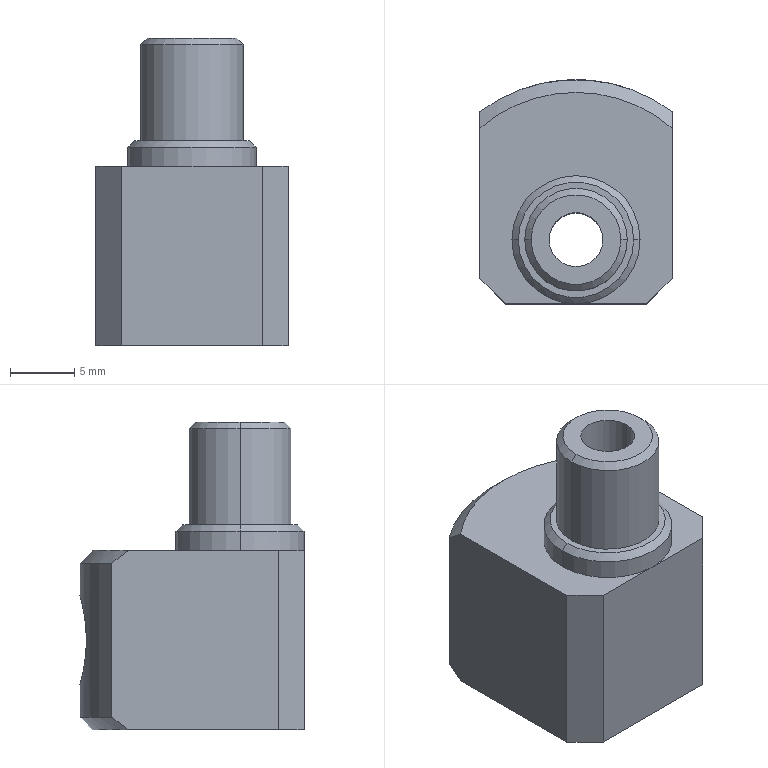Part | SolidWorks | features Chamfer 3, ICE 3, HoleWzd 2, Extrusion 1 | 1 solid | 27 faces | box 15 x 17.5 x 24 mm | volume 3225 mm3 | plane 11 | cylinder 10 | cone 6 | commonest cylinder face diameters 4.2 x3 7 x2 8 x2 10 x2 25 x1
STEP:
#1=CARTESIAN_POINT('',(3.5,0.,12.));
#2=VERTEX_POINT('',#1);
#3=CARTESIAN_POINT('',(-3.5,0.,12.));
#4=VERTEX_POINT('',#3);
#5=CARTESIAN_POINT('',(0.,0.,12.));
#6=DIRECTION('',(0.,0.,1.));
#7=DIRECTION('',(1.,0.,0.));
#8=AXIS2_PLACEMENT_3D('',#5,#6,#7);
#9=CIRCLE('',#8,3.5);
#10=EDGE_CURVE('',#2,#4,#9,.T.);
#11=ORIENTED_EDGE('',*,*,#10,.F.);
#12=CARTESIAN_POINT('',(4.,0.,11.5));
#13=VERTEX_POINT('',#12);
#14=CARTESIAN_POINT('',(3.5,0.,12.));
#15=DIRECTION('',(0.7071,0.,-0.7071));
#16=VECTOR('',#15,1000.);
#17=LINE('',#14,#16);
#18=EDGE_CURVE('',#2,#13,#17,.T.);
#19=ORIENTED_EDGE('',*,*,#18,.T.);
#20=CARTESIAN_POINT('',(-4.,0.,11.5));
#21=VERTEX_POINT('',#20);
#22=CARTESIAN_POINT('',(0.,0.,11.5));
#23=DIRECTION('',(0.,0.,-1.));
#24=DIRECTION('',(1.,0.,0.));
#25=AXIS2_PLACEMENT_3D('',#22,#23,#24);
#26=CIRCLE('',#25,4.);
#27=EDGE_CURVE('',#21,#13,#26,.T.);
#28=ORIENTED_EDGE('',*,*,#27,.F.);
#29=CARTESIAN_POINT('',(-3.5,0.,12.));
#30=DIRECTION('',(-0.7071,0.,-0.7071));
#31=VECTOR('',#30,1000.);
#32=LINE('',#29,#31);
#33=EDGE_CURVE('',#4,#21,#32,.T.);
#34=ORIENTED_EDGE('',*,*,#33,.F.);
#35=EDGE_LOOP('',(#11,#19,#28,#34));
#36=FACE_OUTER_BOUND('',#35,.T.);
#37=CARTESIAN_POINT('',(0.,0.,12.));
#38=DIRECTION('',(0.,0.,-1.));
#39=DIRECTION('',(-1.,0.,0.));
#40=AXIS2_PLACEMENT_3D('',#37,#38,#39);
#41=CONICAL_SURFACE('',#40,3.5,0.7854);
#42=ADVANCED_FACE('',(#36),#41,.T.);
#43=CARTESIAN_POINT('',(4.5,0.,4.));
#44=VERTEX_POINT('',#43);
#45=CARTESIAN_POINT('',(-4.5,0.,4.));
#46=VERTEX_POINT('',#45);
#47=CARTESIAN_POINT('',(0.,0.,4.));
#48=DIRECTION('',(0.,0.,1.));
#49=DIRECTION('',(1.,0.,0.));
#50=AXIS2_PLACEMENT_3D('',#47,#48,#49);
#51=CIRCLE('',#50,4.5);
#52=EDGE_CURVE('',#44,#46,#51,.T.);
#53=ORIENTED_EDGE('',*,*,#52,.F.);
#54=CARTESIAN_POINT('',(5.,0.,3.5));
#55=VERTEX_POINT('',#54);
#56=CARTESIAN_POINT('',(4.5,0.,4.));
#57=DIRECTION('',(0.7071,0.,-0.7071));
#58=VECTOR('',#57,1000.);
#59=LINE('',#56,#58);
#60=EDGE_CURVE('',#44,#55,#59,.T.);
#61=ORIENTED_EDGE('',*,*,#60,.T.);
#62=CARTESIAN_POINT('',(-5.,0.,3.5));
#63=VERTEX_POINT('',#62);
#64=CARTESIAN_POINT('',(0.,0.,3.5));
#65=DIRECTION('',(0.,0.,-1.));
#66=DIRECTION('',(1.,0.,0.));
#67=AXIS2_PLACEMENT_3D('',#64,#65,#66);
#68=CIRCLE('',#67,5.);
#69=EDGE_CURVE('',#63,#55,#68,.T.);
#70=ORIENTED_EDGE('',*,*,#69,.F.);
#71=CARTESIAN_POINT('',(-4.5,0.,4.));
#72=DIRECTION('',(-0.7071,0.,-0.7071));
#73=VECTOR('',#72,1000.);
#74=LINE('',#71,#73);
#75=EDGE_CURVE('',#46,#63,#74,.T.);
#76=ORIENTED_EDGE('',*,*,#75,.F.);
#77=EDGE_LOOP('',(#53,#61,#70,#76));
#78=FACE_OUTER_BOUND('',#77,.T.);
#79=CARTESIAN_POINT('',(0.,0.,4.));
#80=DIRECTION('',(0.,0.,-1.));
#81=DIRECTION('',(-1.,0.,0.));
#82=AXIS2_PLACEMENT_3D('',#79,#80,#81);
#83=CONICAL_SURFACE('',#82,4.5,0.7854);
#84=ADVANCED_FACE('',(#78),#83,.T.);
#85=CARTESIAN_POINT('',(0.,12.5,-1.5));
#86=VERTEX_POINT('',#85);
#87=CARTESIAN_POINT('',(0.,12.5,-8.5));
#88=VERTEX_POINT('',#87);
#89=CARTESIAN_POINT('',(0.,12.5,-1.5));
#90=CARTESIAN_POINT('',(-0.2291,12.5,-1.5));
#91=CARTESIAN_POINT('',(-0.4583,12.494,-1.522));
#92=CARTESIAN_POINT('',(-0.9128,12.469,-1.613));
#93=CARTESIAN_POINT('',(-1.132,12.45,-1.68));
#94=CARTESIAN_POINT('',(-1.553,12.405,-1.855));
#95=CARTESIAN_POINT('',(-1.758,12.377,-1.965));
#96=CARTESIAN_POINT('',(-2.137,12.317,-2.219));
#97=CARTESIAN_POINT('',(-2.313,12.285,-2.363));
#98=CARTESIAN_POINT('',(-2.636,12.22,-2.686));
#99=CARTESIAN_POINT('',(-2.782,12.187,-2.864));
#100=CARTESIAN_POINT('',(-3.035,12.127,-3.242));
#101=CARTESIAN_POINT('',(-3.143,12.099,-3.443));
#102=CARTESIAN_POINT('',(-3.32,12.051,-3.869));
#103=CARTESIAN_POINT('',(-3.387,12.032,-4.088));
#104=CARTESIAN_POINT('',(-3.477,12.007,-4.537));
#105=CARTESIAN_POINT('',(-3.5,12.,-4.769));
#106=CARTESIAN_POINT('',(-3.5,12.,-5.23));
#107=CARTESIAN_POINT('',(-3.477,12.007,-5.458));
#108=CARTESIAN_POINT('',(-3.388,12.032,-5.908));
#109=CARTESIAN_POINT('',(-3.32,12.051,-6.132));
#110=CARTESIAN_POINT('',(-3.145,12.098,-6.553));
#111=CARTESIAN_POINT('',(-3.037,12.126,-6.755));
#112=CARTESIAN_POINT('',(-2.782,12.187,-7.137));
#113=CARTESIAN_POINT('',(-2.636,12.22,-7.313));
#114=CARTESIAN_POINT('',(-2.316,12.285,-7.634));
#115=CARTESIAN_POINT('',(-2.138,12.317,-7.781));
#116=CARTESIAN_POINT('',(-1.757,12.377,-8.035));
#117=CARTESIAN_POINT('',(-1.557,12.404,-8.143));
#118=CARTESIAN_POINT('',(-1.135,12.45,-8.319));
#119=CARTESIAN_POINT('',(-0.9118,12.469,-8.387));
#120=CARTESIAN_POINT('',(-0.4613,12.494,-8.477));
#121=CARTESIAN_POINT('',(-0.2324,12.5,-8.5));
#122=CARTESIAN_POINT('',(0.,12.5,-8.5));
#123=B_SPLINE_CURVE_WITH_KNOTS('',3,(#89,#90,#91,#92,#93,#94,#95,#96,#97,#98,#99,#100,#101,#102,#103,#104,#105,#106,#107,#108,#109,#110,#111,#112,#113,#114,#115,#116,#117,#118,#119,#120,#121,#122),.UNSPECIFIED.,.F.,.F.,(4,2,2,2,2,2,2,2,2,2,2,2,2,2,2,2,4),(0.011,0.01169,0.01237,0.01306,0.01375,0.01443,0.01512,0.01581,0.0165,0.01718,0.01787,0.01856,0.01924,0.01993,0.02062,0.02131,0.02199),.UNSPECIFIED.);
#124=EDGE_CURVE('',#86,#88,#123,.T.);
#125=ORIENTED_EDGE('',*,*,#124,.F.);
#126=CARTESIAN_POINT('',(0.,2.1,-1.5));
#127=VERTEX_POINT('',#126);
#128=CARTESIAN_POINT('',(0.,0.,-1.5));
#129=DIRECTION('',(0.,-1.,0.));
#130=VECTOR('',#129,1000.);
#131=LINE('',#128,#130);
#132=EDGE_CURVE('',#86,#127,#131,.T.);
#133=ORIENTED_EDGE('',*,*,#132,.T.);
#134=CARTESIAN_POINT('',(-2.1,0.,-2.2));
#135=VERTEX_POINT('',#134);
#136=CARTESIAN_POINT('',(-2.1,0.,-2.2));
#137=CARTESIAN_POINT('',(-2.1,0.1429,-2.2));
#138=CARTESIAN_POINT('',(-2.086,0.2824,-2.189));
#139=CARTESIAN_POINT('',(-2.03,0.5553,-2.149));
#140=CARTESIAN_POINT('',(-1.988,0.6898,-2.119));
#141=CARTESIAN_POINT('',(-1.829,1.068,-2.013));
#142=CARTESIAN_POINT('',(-1.675,1.294,-1.92));
#143=CARTESIAN_POINT('',(-1.392,1.578,-1.787));
#144=CARTESIAN_POINT('',(-1.287,1.665,-1.743));
#145=CARTESIAN_POINT('',(-1.062,1.816,-1.663));
#146=CARTESIAN_POINT('',(-0.9435,1.881,-1.627));
#147=CARTESIAN_POINT('',(-0.6905,1.988,-1.566));
#148=CARTESIAN_POINT('',(-0.5548,2.03,-1.542));
#149=CARTESIAN_POINT('',(-0.2811,2.086,-1.509));
#150=CARTESIAN_POINT('',(-0.1418,2.1,-1.5));
#151=CARTESIAN_POINT('',(0.,2.1,-1.5));
#152=B_SPLINE_CURVE_WITH_KNOTS('',3,(#136,#137,#138,#139,#140,#141,#142,#143,#144,#145,#146,#147,#148,#149,#150,#151),.UNSPECIFIED.,.F.,.F.,(4,2,2,2,2,2,2,4),(0.,0.0004214,0.0008428,0.001686,0.002107,0.002528,0.00295,0.003371),.UNSPECIFIED.);
#153=EDGE_CURVE('',#135,#127,#152,.T.);
#154=ORIENTED_EDGE('',*,*,#153,.F.);
#155=CARTESIAN_POINT('',(-2.1,0.,-7.8));
#156=VERTEX_POINT('',#155);
#157=CARTESIAN_POINT('',(0.,0.,-5.));
#158=DIRECTION('',(0.,-1.,0.));
#159=DIRECTION('',(0.,0.,-1.));
#160=AXIS2_PLACEMENT_3D('',#157,#158,#159);
#161=CIRCLE('',#160,3.5);
#162=EDGE_CURVE('',#135,#156,#161,.T.);
#163=ORIENTED_EDGE('',*,*,#162,.T.);
#164=CARTESIAN_POINT('',(0.,2.1,-8.5));
#165=VERTEX_POINT('',#164);
#166=CARTESIAN_POINT('',(0.,2.1,-8.5));
#167=CARTESIAN_POINT('',(-0.2831,2.1,-8.5));
#168=CARTESIAN_POINT('',(-0.5647,2.041,-8.464));
#169=CARTESIAN_POINT('',(-1.073,1.826,-8.342));
#170=CARTESIAN_POINT('',(-1.3,1.671,-8.256));
#171=CARTESIAN_POINT('',(-1.583,1.387,-8.123));
#172=CARTESIAN_POINT('',(-1.669,1.282,-8.078));
#173=CARTESIAN_POINT('',(-1.819,1.059,-7.992));
#174=CARTESIAN_POINT('',(-1.882,0.9407,-7.951));
#175=CARTESIAN_POINT('',(-1.988,0.6903,-7.881));
#176=CARTESIAN_POINT('',(-2.03,0.556,-7.851));
#177=CARTESIAN_POINT('',(-2.086,0.2824,-7.811));
#178=CARTESIAN_POINT('',(-2.1,0.1428,-7.8));
#179=CARTESIAN_POINT('',(-2.1,0.,-7.8));
#180=B_SPLINE_CURVE_WITH_KNOTS('',3,(#166,#167,#168,#169,#170,#171,#172,#173,#174,#175,#176,#177,#178,#179),.UNSPECIFIED.,.F.,.F.,(4,2,2,2,2,2,4),(0.003371,0.004212,0.005053,0.005473,0.005894,0.006314,0.006735),.UNSPECIFIED.);
#181=EDGE_CURVE('',#165,#156,#180,.T.);
#182=ORIENTED_EDGE('',*,*,#181,.F.);
#183=CARTESIAN_POINT('',(0.,0.,-8.5));
#184=DIRECTION('',(0.,-1.,0.));
#185=VECTOR('',#184,1000.);
#186=LINE('',#183,#185);
#187=EDGE_CURVE('',#88,#165,#186,.T.);
#188=ORIENTED_EDGE('',*,*,#187,.F.);
#189=EDGE_LOOP('',(#125,#133,#154,#163,#182,#188));
#190=FACE_OUTER_BOUND('',#189,.T.);
#191=CARTESIAN_POINT('',(0.,0.,-5.));
#192=DIRECTION('',(0.,-1.,0.));
#193=DIRECTION('',(0.,0.,-1.));
#194=AXIS2_PLACEMENT_3D('',#191,#192,#193);
#195=CYLINDRICAL_SURFACE('',#194,3.5);
#196=ADVANCED_FACE('',(#190),#195,.F.);
#197=ORIENTED_EDGE('',*,*,#69,.T.);
#198=CARTESIAN_POINT('',(5.,0.,2.));
#199=VERTEX_POINT('',#198);
#200=CARTESIAN_POINT('',(5.,0.,4.));
#201=DIRECTION('',(0.,0.,-1.));
#202=VECTOR('',#201,1000.);
#203=LINE('',#200,#202);
#204=EDGE_CURVE('',#55,#199,#203,.T.);
#205=ORIENTED_EDGE('',*,*,#204,.T.);
#206=CARTESIAN_POINT('',(-5.,0.,2.));
#207=VERTEX_POINT('',#206);
#208=CARTESIAN_POINT('',(0.,0.,2.));
#209=DIRECTION('',(0.,0.,1.));
#210=DIRECTION('',(1.,0.,0.));
#211=AXIS2_PLACEMENT_3D('',#208,#209,#210);
#212=CIRCLE('',#211,5.);
#213=EDGE_CURVE('',#199,#207,#212,.T.);
#214=ORIENTED_EDGE('',*,*,#213,.T.);
#215=CARTESIAN_POINT('',(-5.,0.,4.));
#216=DIRECTION('',(0.,0.,-1.));
#217=VECTOR('',#216,1000.);
#218=LINE('',#215,#217);
#219=EDGE_CURVE('',#63,#207,#218,.T.);
#220=ORIENTED_EDGE('',*,*,#219,.F.);
#221=EDGE_LOOP('',(#197,#205,#214,#220));
#222=FACE_OUTER_BOUND('',#221,.T.);
#223=CARTESIAN_POINT('',(0.,0.,4.));
#224=DIRECTION('',(0.,0.,-1.));
#225=DIRECTION('',(-1.,0.,0.));
#226=AXIS2_PLACEMENT_3D('',#223,#224,#225);
#227=CYLINDRICAL_SURFACE('',#226,5.);
#228=ADVANCED_FACE('',(#222),#227,.T.);
#229=CARTESIAN_POINT('',(2.1,0.,12.));
#230=VERTEX_POINT('',#229);
#231=CARTESIAN_POINT('',(-2.1,0.,12.));
#232=VERTEX_POINT('',#231);
#233=CARTESIAN_POINT('',(0.,0.,12.));
#234=DIRECTION('',(0.,0.,-1.));
#235=DIRECTION('',(-1.,0.,0.));
#236=AXIS2_PLACEMENT_3D('',#233,#234,#235);
#237=CIRCLE('',#236,2.1);
#238=EDGE_CURVE('',#230,#232,#237,.T.);
#239=ORIENTED_EDGE('',*,*,#238,.F.);
#240=CARTESIAN_POINT('',(2.1,0.,-2.2));
#241=VERTEX_POINT('',#240);
#242=CARTESIAN_POINT('',(2.1,0.,-12.));
#243=DIRECTION('',(0.,0.,-1.));
#244=VECTOR('',#243,1000.);
#245=LINE('',#242,#244);
#246=EDGE_CURVE('',#230,#241,#245,.T.);
#247=ORIENTED_EDGE('',*,*,#246,.T.);
#248=CARTESIAN_POINT('',(2.1,0.,-7.8));
#249=VERTEX_POINT('',#248);
#250=CARTESIAN_POINT('',(2.1,0.,-12.));
#251=DIRECTION('',(0.,0.,-1.));
#252=VECTOR('',#251,1000.);
#253=LINE('',#250,#252);
#254=EDGE_CURVE('',#241,#249,#253,.T.);
#255=ORIENTED_EDGE('',*,*,#254,.T.);
#256=CARTESIAN_POINT('',(2.1,0.,-12.));
#257=VERTEX_POINT('',#256);
#258=CARTESIAN_POINT('',(2.1,0.,-12.));
#259=DIRECTION('',(0.,0.,-1.));
#260=VECTOR('',#259,1000.);
#261=LINE('',#258,#260);
#262=EDGE_CURVE('',#249,#257,#261,.T.);
#263=ORIENTED_EDGE('',*,*,#262,.T.);
#264=CARTESIAN_POINT('',(-2.1,0.,-12.));
#265=VERTEX_POINT('',#264);
#266=CARTESIAN_POINT('',(0.,0.,-12.));
#267=DIRECTION('',(0.,0.,-1.));
#268=DIRECTION('',(-1.,0.,0.));
#269=AXIS2_PLACEMENT_3D('',#266,#267,#268);
#270=CIRCLE('',#269,2.1);
#271=EDGE_CURVE('',#257,#265,#270,.T.);
#272=ORIENTED_EDGE('',*,*,#271,.T.);
#273=CARTESIAN_POINT('',(-2.1,0.,-12.));
#274=DIRECTION('',(0.,0.,-1.));
#275=VECTOR('',#274,1000.);
#276=LINE('',#273,#275);
#277=EDGE_CURVE('',#156,#265,#276,.T.);
#278=ORIENTED_EDGE('',*,*,#277,.F.);
#279=CARTESIAN_POINT('',(-2.1,0.,-12.));
#280=DIRECTION('',(0.,0.,1.));
#281=VECTOR('',#280,1000.);
#282=LINE('',#279,#281);
#283=EDGE_CURVE('',#156,#135,#282,.T.);
#284=ORIENTED_EDGE('',*,*,#283,.T.);
#285=CARTESIAN_POINT('',(-2.1,0.,-12.));
#286=DIRECTION('',(0.,0.,-1.));
#287=VECTOR('',#286,1000.);
#288=LINE('',#285,#287);
#289=EDGE_CURVE('',#232,#135,#288,.T.);
#290=ORIENTED_EDGE('',*,*,#289,.F.);
#291=EDGE_LOOP('',(#239,#247,#255,#263,#272,#278,#284,#290));
#292=FACE_OUTER_BOUND('',#291,.T.);
#293=CARTESIAN_POINT('',(0.,0.,-12.));
#294=DIRECTION('',(0.,0.,-1.));
#295=DIRECTION('',(-1.,0.,0.));
#296=AXIS2_PLACEMENT_3D('',#293,#294,#295);
#297=CYLINDRICAL_SURFACE('',#296,2.1);
#298=ADVANCED_FACE('',(#292),#297,.F.);
#299=ORIENTED_EDGE('',*,*,#246,.F.);
#300=CARTESIAN_POINT('',(0.,0.,12.));
#301=DIRECTION('',(0.,0.,-1.));
#302=DIRECTION('',(-1.,0.,0.));
#303=AXIS2_PLACEMENT_3D('',#300,#301,#302);
#304=CIRCLE('',#303,2.1);
#305=EDGE_CURVE('',#232,#230,#304,.T.);
#306=ORIENTED_EDGE('',*,*,#305,.F.);
#307=ORIENTED_EDGE('',*,*,#289,.T.);
#308=ORIENTED_EDGE('',*,*,#153,.T.);
#309=CARTESIAN_POINT('',(0.,2.1,-1.5));
#310=CARTESIAN_POINT('',(0.2831,2.1,-1.5));
#311=CARTESIAN_POINT('',(0.5647,2.041,-1.536));
#312=CARTESIAN_POINT('',(1.073,1.826,-1.658));
#313=CARTESIAN_POINT('',(1.3,1.671,-1.744));
#314=CARTESIAN_POINT('',(1.583,1.387,-1.877));
#315=CARTESIAN_POINT('',(1.669,1.282,-1.922));
#316=CARTESIAN_POINT('',(1.819,1.059,-2.008));
#317=CARTESIAN_POINT('',(1.882,0.9407,-2.049));
#318=CARTESIAN_POINT('',(1.988,0.6903,-2.119));
#319=CARTESIAN_POINT('',(2.03,0.556,-2.149));
#320=CARTESIAN_POINT('',(2.086,0.2824,-2.189));
#321=CARTESIAN_POINT('',(2.1,0.1428,-2.2));
#322=CARTESIAN_POINT('',(2.1,0.,-2.2));
#323=B_SPLINE_CURVE_WITH_KNOTS('',3,(#309,#310,#311,#312,#313,#314,#315,#316,#317,#318,#319,#320,#321,#322),.UNSPECIFIED.,.F.,.F.,(4,2,2,2,2,2,4),(0.003371,0.004212,0.005053,0.005473,0.005894,0.006314,0.006735),.UNSPECIFIED.);
#324=EDGE_CURVE('',#127,#241,#323,.T.);
#325=ORIENTED_EDGE('',*,*,#324,.T.);
#326=EDGE_LOOP('',(#299,#306,#307,#308,#325));
#327=FACE_OUTER_BOUND('',#326,.T.);
#328=CARTESIAN_POINT('',(0.,0.,-12.));
#329=DIRECTION('',(0.,0.,-1.));
#330=DIRECTION('',(-1.,0.,0.));
#331=AXIS2_PLACEMENT_3D('',#328,#329,#330);
#332=CYLINDRICAL_SURFACE('',#331,2.1);
#333=ADVANCED_FACE('',(#327),#332,.F.);
#334=CARTESIAN_POINT('',(-4.,0.,4.));
#335=VERTEX_POINT('',#334);
#336=CARTESIAN_POINT('',(4.,0.,4.));
#337=VERTEX_POINT('',#336);
#338=CARTESIAN_POINT('',(0.,0.,4.));
#339=DIRECTION('',(0.,0.,-1.));
#340=DIRECTION('',(1.,0.,0.));
#341=AXIS2_PLACEMENT_3D('',#338,#339,#340);
#342=CIRCLE('',#341,4.);
#343=EDGE_CURVE('',#335,#337,#342,.T.);
#344=ORIENTED_EDGE('',*,*,#343,.F.);
#345=CARTESIAN_POINT('',(-4.,0.,2.));
#346=DIRECTION('',(0.,0.,1.));
#347=VECTOR('',#346,1000.);
#348=LINE('',#345,#347);
#349=EDGE_CURVE('',#335,#21,#348,.T.);
#350=ORIENTED_EDGE('',*,*,#349,.T.);
#351=ORIENTED_EDGE('',*,*,#27,.T.);
#352=CARTESIAN_POINT('',(4.,0.,2.));
#353=DIRECTION('',(0.,0.,1.));
#354=VECTOR('',#353,1000.);
#355=LINE('',#352,#354);
#356=EDGE_CURVE('',#337,#13,#355,.T.);
#357=ORIENTED_EDGE('',*,*,#356,.F.);
#358=EDGE_LOOP('',(#344,#350,#351,#357));
#359=FACE_OUTER_BOUND('',#358,.T.);
#360=CARTESIAN_POINT('',(0.,0.,2.));
#361=DIRECTION('',(0.,0.,1.));
#362=DIRECTION('',(1.,0.,0.));
#363=AXIS2_PLACEMENT_3D('',#360,#361,#362);
#364=CYLINDRICAL_SURFACE('',#363,4.);
#365=ADVANCED_FACE('',(#359),#364,.T.);
#366=CARTESIAN_POINT('',(7.5,-3.,2.));
#367=VERTEX_POINT('',#366);
#368=CARTESIAN_POINT('',(7.5,8.718,2.));
#369=VERTEX_POINT('',#368);
#370=CARTESIAN_POINT('',(7.5,0.,2.));
#371=DIRECTION('',(0.,1.,0.));
#372=VECTOR('',#371,1000.);
#373=LINE('',#370,#372);
#374=EDGE_CURVE('',#367,#369,#373,.T.);
#375=ORIENTED_EDGE('',*,*,#374,.T.);
#376=CARTESIAN_POINT('',(-7.5,8.718,2.));
#377=VERTEX_POINT('',#376);
#378=CARTESIAN_POINT('',(0.,0.,2.));
#379=DIRECTION('',(0.,0.,1.));
#380=DIRECTION('',(1.,0.,0.));
#381=AXIS2_PLACEMENT_3D('',#378,#379,#380);
#382=CIRCLE('',#381,11.5);
#383=EDGE_CURVE('',#369,#377,#382,.T.);
#384=ORIENTED_EDGE('',*,*,#383,.T.);
#385=CARTESIAN_POINT('',(-7.5,-3.,2.));
#386=VERTEX_POINT('',#385);
#387=CARTESIAN_POINT('',(-7.5,0.,2.));
#388=DIRECTION('',(0.,-1.,0.));
#389=VECTOR('',#388,1000.);
#390=LINE('',#387,#389);
#391=EDGE_CURVE('',#377,#386,#390,.T.);
#392=ORIENTED_EDGE('',*,*,#391,.T.);
#393=CARTESIAN_POINT('',(-5.5,-5.,2.));
#394=VERTEX_POINT('',#393);
#395=CARTESIAN_POINT('',(-5.25,-5.25,2.));
#396=DIRECTION('',(0.7071,-0.7071,0.));
#397=VECTOR('',#396,1000.);
#398=LINE('',#395,#397);
#399=EDGE_CURVE('',#386,#394,#398,.T.);
#400=ORIENTED_EDGE('',*,*,#399,.T.);
#401=CARTESIAN_POINT('',(0.,-5.,2.));
#402=VERTEX_POINT('',#401);
#403=CARTESIAN_POINT('',(0.,-5.,2.));
#404=DIRECTION('',(1.,0.,0.));
#405=VECTOR('',#404,1000.);
#406=LINE('',#403,#405);
#407=EDGE_CURVE('',#394,#402,#406,.T.);
#408=ORIENTED_EDGE('',*,*,#407,.T.);
#409=CARTESIAN_POINT('',(0.,0.,2.));
#410=DIRECTION('',(0.,0.,1.));
#411=DIRECTION('',(1.,0.,0.));
#412=AXIS2_PLACEMENT_3D('',#409,#410,#411);
#413=CIRCLE('',#412,5.);
#414=EDGE_CURVE('',#207,#402,#413,.T.);
#415=ORIENTED_EDGE('',*,*,#414,.F.);
#416=ORIENTED_EDGE('',*,*,#213,.F.);
#417=CARTESIAN_POINT('',(0.,0.,2.));
#418=DIRECTION('',(0.,0.,1.));
#419=DIRECTION('',(1.,0.,0.));
#420=AXIS2_PLACEMENT_3D('',#417,#418,#419);
#421=CIRCLE('',#420,5.);
#422=EDGE_CURVE('',#402,#199,#421,.T.);
#423=ORIENTED_EDGE('',*,*,#422,.F.);
#424=CARTESIAN_POINT('',(5.5,-5.,2.));
#425=VERTEX_POINT('',#424);
#426=CARTESIAN_POINT('',(0.,-5.,2.));
#427=DIRECTION('',(1.,0.,0.));
#428=VECTOR('',#427,1000.);
#429=LINE('',#426,#428);
#430=EDGE_CURVE('',#402,#425,#429,.T.);
#431=ORIENTED_EDGE('',*,*,#430,.T.);
#432=CARTESIAN_POINT('',(5.25,-5.25,2.));
#433=DIRECTION('',(0.7071,0.7071,0.));
#434=VECTOR('',#433,1000.);
#435=LINE('',#432,#434);
#436=EDGE_CURVE('',#425,#367,#435,.T.);
#437=ORIENTED_EDGE('',*,*,#436,.T.);
#438=EDGE_LOOP('',(#375,#384,#392,#400,#408,#415,#416,#423,#431,#437));
#439=FACE_OUTER_BOUND('',#438,.T.);
#440=CARTESIAN_POINT('',(0.,0.,2.));
#441=DIRECTION('',(0.,0.,1.));
#442=DIRECTION('',(1.,0.,0.));
#443=AXIS2_PLACEMENT_3D('',#440,#441,#442);
#444=PLANE('',#443);
#445=ADVANCED_FACE('',(#439),#444,.T.);
#446=CARTESIAN_POINT('',(0.,12.5,-8.5));
#447=CARTESIAN_POINT('',(0.2325,12.5,-8.5));
#448=CARTESIAN_POINT('',(0.4609,12.494,-8.477));
#449=CARTESIAN_POINT('',(0.9099,12.469,-8.387));
#450=CARTESIAN_POINT('',(1.133,12.45,-8.32));
#451=CARTESIAN_POINT('',(1.556,12.405,-8.143));
#452=CARTESIAN_POINT('',(1.757,12.377,-8.036));
#453=CARTESIAN_POINT('',(2.136,12.318,-7.782));
#454=CARTESIAN_POINT('',(2.315,12.285,-7.635));
#455=CARTESIAN_POINT('',(2.636,12.22,-7.313));
#456=CARTESIAN_POINT('',(2.781,12.187,-7.138));
#457=CARTESIAN_POINT('',(3.037,12.126,-6.756));
#458=CARTESIAN_POINT('',(3.144,12.098,-6.554));
#459=CARTESIAN_POINT('',(3.319,12.052,-6.133));
#460=CARTESIAN_POINT('',(3.387,12.032,-5.911));
#461=CARTESIAN_POINT('',(3.477,12.007,-5.459));
#462=CARTESIAN_POINT('',(3.5,12.,-5.231));
#463=CARTESIAN_POINT('',(3.5,12.,-4.772));
#464=CARTESIAN_POINT('',(3.477,12.007,-4.539));
#465=CARTESIAN_POINT('',(3.387,12.032,-4.089));
#466=CARTESIAN_POINT('',(3.321,12.051,-3.87));
#467=CARTESIAN_POINT('',(3.144,12.099,-3.445));
#468=CARTESIAN_POINT('',(3.035,12.127,-3.242));
#469=CARTESIAN_POINT('',(2.782,12.187,-2.864));
#470=CARTESIAN_POINT('',(2.636,12.22,-2.686));
#471=CARTESIAN_POINT('',(2.312,12.285,-2.363));
#472=CARTESIAN_POINT('',(2.137,12.317,-2.219));
#473=CARTESIAN_POINT('',(1.759,12.377,-1.965));
#474=CARTESIAN_POINT('',(1.554,12.405,-1.855));
#475=CARTESIAN_POINT('',(1.131,12.451,-1.68));
#476=CARTESIAN_POINT('',(0.913,12.469,-1.613));
#477=CARTESIAN_POINT('',(0.4615,12.494,-1.523));
#478=CARTESIAN_POINT('',(0.2291,12.5,-1.5));
#479=CARTESIAN_POINT('',(0.,12.5,-1.5));
#480=B_SPLINE_CURVE_WITH_KNOTS('',3,(#446,#447,#448,#449,#450,#451,#452,#453,#454,#455,#456,#457,#458,#459,#460,#461,#462,#463,#464,#465,#466,#467,#468,#469,#470,#471,#472,#473,#474,#475,#476,#477,#478,#479),.UNSPECIFIED.,.F.,.F.,(4,2,2,2,2,2,2,2,2,2,2,2,2,2,2,2,4),(0.,0.0006874,0.001375,0.002062,0.002749,0.003437,0.004124,0.004812,0.005499,0.006186,0.006874,0.007561,0.008248,0.008936,0.009623,0.01031,0.011),.UNSPECIFIED.);
#481=EDGE_CURVE('',#88,#86,#480,.T.);
#482=ORIENTED_EDGE('',*,*,#481,.T.);
#483=ORIENTED_EDGE('',*,*,#124,.T.);
#484=EDGE_LOOP('',(#482,#483));
#485=FACE_BOUND('',#484,.T.);
#486=CARTESIAN_POINT('',(-7.5,10.,1.));
#487=VERTEX_POINT('',#486);
#488=CARTESIAN_POINT('',(-7.5,10.,-11.));
#489=VERTEX_POINT('',#488);
#490=CARTESIAN_POINT('',(-7.5,10.,12.));
#491=DIRECTION('',(0.,0.,-1.));
#492=VECTOR('',#491,1000.);
#493=LINE('',#490,#492);
#494=EDGE_CURVE('',#487,#489,#493,.T.);
#495=ORIENTED_EDGE('',*,*,#494,.F.);
#496=CARTESIAN_POINT('',(7.5,10.,1.));
#497=VERTEX_POINT('',#496);
#498=CARTESIAN_POINT('',(0.,0.,1.));
#499=DIRECTION('',(0.,0.,-1.));
#500=DIRECTION('',(1.,0.,0.));
#501=AXIS2_PLACEMENT_3D('',#498,#499,#500);
#502=CIRCLE('',#501,12.5);
#503=EDGE_CURVE('',#487,#497,#502,.T.);
#504=ORIENTED_EDGE('',*,*,#503,.T.);
#505=CARTESIAN_POINT('',(7.5,10.,-11.));
#506=VERTEX_POINT('',#505);
#507=CARTESIAN_POINT('',(7.5,10.,12.));
#508=DIRECTION('',(0.,0.,1.));
#509=VECTOR('',#508,1000.);
#510=LINE('',#507,#509);
#511=EDGE_CURVE('',#506,#497,#510,.T.);
#512=ORIENTED_EDGE('',*,*,#511,.F.);
#513=CARTESIAN_POINT('',(0.,0.,-11.));
#514=DIRECTION('',(0.,0.,1.));
#515=DIRECTION('',(1.,0.,0.));
#516=AXIS2_PLACEMENT_3D('',#513,#514,#515);
#517=CIRCLE('',#516,12.5);
#518=EDGE_CURVE('',#506,#489,#517,.T.);
#519=ORIENTED_EDGE('',*,*,#518,.T.);
#520=EDGE_LOOP('',(#495,#504,#512,#519));
#521=FACE_OUTER_BOUND('',#520,.T.);
#522=CARTESIAN_POINT('',(0.,0.,12.));
#523=DIRECTION('',(0.,0.,-1.));
#524=DIRECTION('',(-1.,0.,0.));
#525=AXIS2_PLACEMENT_3D('',#522,#523,#524);
#526=CYLINDRICAL_SURFACE('',#525,12.5);
#527=ADVANCED_FACE('',(#485,#521),#526,.T.);
#528=CARTESIAN_POINT('',(0.,0.,-12.));
#529=DIRECTION('',(0.,0.,-1.));
#530=DIRECTION('',(-1.,0.,0.));
#531=AXIS2_PLACEMENT_3D('',#528,#529,#530);
#532=CIRCLE('',#531,2.1);
#533=EDGE_CURVE('',#265,#257,#532,.T.);
#534=ORIENTED_EDGE('',*,*,#533,.F.);
#535=ORIENTED_EDGE('',*,*,#271,.F.);
#536=EDGE_LOOP('',(#534,#535));
#537=FACE_BOUND('',#536,.T.);
#538=CARTESIAN_POINT('',(-7.5,-3.,-12.));
#539=VERTEX_POINT('',#538);
#540=CARTESIAN_POINT('',(-7.5,8.718,-12.));
#541=VERTEX_POINT('',#540);
#542=CARTESIAN_POINT('',(-7.5,15.,-12.));
#543=DIRECTION('',(0.,1.,0.));
#544=VECTOR('',#543,1000.);
#545=LINE('',#542,#544);
#546=EDGE_CURVE('',#539,#541,#545,.T.);
#547=ORIENTED_EDGE('',*,*,#546,.T.);
#548=CARTESIAN_POINT('',(7.5,8.718,-12.));
#549=VERTEX_POINT('',#548);
#550=CARTESIAN_POINT('',(0.,0.,-12.));
#551=DIRECTION('',(0.,0.,-1.));
#552=DIRECTION('',(1.,0.,0.));
#553=AXIS2_PLACEMENT_3D('',#550,#551,#552);
#554=CIRCLE('',#553,11.5);
#555=EDGE_CURVE('',#541,#549,#554,.T.);
#556=ORIENTED_EDGE('',*,*,#555,.T.);
#557=CARTESIAN_POINT('',(7.5,-3.,-12.));
#558=VERTEX_POINT('',#557);
#559=CARTESIAN_POINT('',(7.5,15.,-12.));
#560=DIRECTION('',(0.,-1.,0.));
#561=VECTOR('',#560,1000.);
#562=LINE('',#559,#561);
#563=EDGE_CURVE('',#549,#558,#562,.T.);
#564=ORIENTED_EDGE('',*,*,#563,.T.);
#565=CARTESIAN_POINT('',(5.5,-5.,-12.));
#566=VERTEX_POINT('',#565);
#567=CARTESIAN_POINT('',(7.5,-3.,-12.));
#568=DIRECTION('',(-0.7071,-0.7071,0.));
#569=VECTOR('',#568,1000.);
#570=LINE('',#567,#569);
#571=EDGE_CURVE('',#558,#566,#570,.T.);
#572=ORIENTED_EDGE('',*,*,#571,.T.);
#573=CARTESIAN_POINT('',(-5.5,-5.,-12.));
#574=VERTEX_POINT('',#573);
#575=CARTESIAN_POINT('',(7.5,-5.,-12.));
#576=DIRECTION('',(-1.,0.,0.));
#577=VECTOR('',#576,1000.);
#578=LINE('',#575,#577);
#579=EDGE_CURVE('',#566,#574,#578,.T.);
#580=ORIENTED_EDGE('',*,*,#579,.T.);
#581=CARTESIAN_POINT('',(-5.5,-5.,-12.));
#582=DIRECTION('',(-0.7071,0.7071,0.));
#583=VECTOR('',#582,1000.);
#584=LINE('',#581,#583);
#585=EDGE_CURVE('',#574,#539,#584,.T.);
#586=ORIENTED_EDGE('',*,*,#585,.T.);
#587=EDGE_LOOP('',(#547,#556,#564,#572,#580,#586));
#588=FACE_OUTER_BOUND('',#587,.T.);
#589=CARTESIAN_POINT('',(0.,0.,-12.));
#590=DIRECTION('',(0.,0.,1.));
#591=DIRECTION('',(1.,0.,0.));
#592=AXIS2_PLACEMENT_3D('',#589,#590,#591);
#593=PLANE('',#592);
#594=ADVANCED_FACE('',(#537,#588),#593,.F.);
#595=ORIENTED_EDGE('',*,*,#349,.F.);
#596=CARTESIAN_POINT('',(0.,0.,4.));
#597=DIRECTION('',(0.,0.,-1.));
#598=DIRECTION('',(1.,0.,0.));
#599=AXIS2_PLACEMENT_3D('',#596,#597,#598);
#600=CIRCLE('',#599,4.);
#601=EDGE_CURVE('',#337,#335,#600,.T.);
#602=ORIENTED_EDGE('',*,*,#601,.F.);
#603=ORIENTED_EDGE('',*,*,#356,.T.);
#604=CARTESIAN_POINT('',(0.,0.,11.5));
#605=DIRECTION('',(0.,0.,-1.));
#606=DIRECTION('',(1.,0.,0.));
#607=AXIS2_PLACEMENT_3D('',#604,#605,#606);
#608=CIRCLE('',#607,4.);
#609=EDGE_CURVE('',#13,#21,#608,.T.);
#610=ORIENTED_EDGE('',*,*,#609,.T.);
#611=EDGE_LOOP('',(#595,#602,#603,#610));
#612=FACE_OUTER_BOUND('',#611,.T.);
#613=CARTESIAN_POINT('',(0.,0.,2.));
#614=DIRECTION('',(0.,0.,1.));
#615=DIRECTION('',(1.,0.,0.));
#616=AXIS2_PLACEMENT_3D('',#613,#614,#615);
#617=CYLINDRICAL_SURFACE('',#616,4.);
#618=ADVANCED_FACE('',(#612),#617,.T.);
#619=CARTESIAN_POINT('',(0.,0.,12.));
#620=DIRECTION('',(0.,0.,1.));
#621=DIRECTION('',(1.,0.,0.));
#622=AXIS2_PLACEMENT_3D('',#619,#620,#621);
#623=CIRCLE('',#622,3.5);
#624=EDGE_CURVE('',#4,#2,#623,.T.);
#625=ORIENTED_EDGE('',*,*,#624,.T.);
#626=ORIENTED_EDGE('',*,*,#10,.T.);
#627=EDGE_LOOP('',(#625,#626));
#628=FACE_OUTER_BOUND('',#627,.T.);
#629=ORIENTED_EDGE('',*,*,#305,.T.);
#630=ORIENTED_EDGE('',*,*,#238,.T.);
#631=EDGE_LOOP('',(#629,#630));
#632=FACE_BOUND('',#631,.T.);
#633=CARTESIAN_POINT('',(0.,0.,12.));
#634=DIRECTION('',(0.,0.,1.));
#635=DIRECTION('',(1.,0.,0.));
#636=AXIS2_PLACEMENT_3D('',#633,#634,#635);
#637=PLANE('',#636);
#638=ADVANCED_FACE('',(#628,#632),#637,.T.);
#639=ORIENTED_EDGE('',*,*,#511,.T.);
#640=CARTESIAN_POINT('',(7.5,10.,1.));
#641=CARTESIAN_POINT('',(7.5,9.577,1.339));
#642=CARTESIAN_POINT('',(7.5,9.15,1.673));
#643=CARTESIAN_POINT('',(7.5,8.718,2.));
#644=B_SPLINE_CURVE_WITH_KNOTS('',3,(#640,#641,#642,#643),.UNSPECIFIED.,.F.,.F.,(4,4),(0.,0.001626),.UNSPECIFIED.);
#645=EDGE_CURVE('',#497,#369,#644,.T.);
#646=ORIENTED_EDGE('',*,*,#645,.T.);
#647=ORIENTED_EDGE('',*,*,#374,.F.);
#648=CARTESIAN_POINT('',(7.5,-3.,12.));
#649=DIRECTION('',(0.,0.,-1.));
#650=VECTOR('',#649,1000.);
#651=LINE('',#648,#650);
#652=EDGE_CURVE('',#367,#558,#651,.T.);
#653=ORIENTED_EDGE('',*,*,#652,.T.);
#654=ORIENTED_EDGE('',*,*,#563,.F.);
#655=CARTESIAN_POINT('',(7.5,8.718,-12.));
#656=CARTESIAN_POINT('',(7.5,9.15,-11.673));
#657=CARTESIAN_POINT('',(7.5,9.577,-11.339));
#658=CARTESIAN_POINT('',(7.5,10.,-11.));
#659=B_SPLINE_CURVE_WITH_KNOTS('',3,(#655,#656,#657,#658),.UNSPECIFIED.,.F.,.F.,(4,4),(0.,0.001626),.UNSPECIFIED.);
#660=EDGE_CURVE('',#549,#506,#659,.T.);
#661=ORIENTED_EDGE('',*,*,#660,.T.);
#662=EDGE_LOOP('',(#639,#646,#647,#653,#654,#661));
#663=FACE_OUTER_BOUND('',#662,.T.);
#664=CARTESIAN_POINT('',(7.5,15.,12.));
#665=DIRECTION('',(1.,0.,0.));
#666=DIRECTION('',(0.,1.,0.));
#667=AXIS2_PLACEMENT_3D('',#664,#665,#666);
#668=PLANE('',#667);
#669=ADVANCED_FACE('',(#663),#668,.T.);
#670=ORIENTED_EDGE('',*,*,#391,.F.);
#671=CARTESIAN_POINT('',(-7.5,8.718,2.));
#672=CARTESIAN_POINT('',(-7.5,9.15,1.673));
#673=CARTESIAN_POINT('',(-7.5,9.577,1.339));
#674=CARTESIAN_POINT('',(-7.5,10.,1.));
#675=B_SPLINE_CURVE_WITH_KNOTS('',3,(#671,#672,#673,#674),.UNSPECIFIED.,.F.,.F.,(4,4),(0.,0.001626),.UNSPECIFIED.);
#676=EDGE_CURVE('',#377,#487,#675,.T.);
#677=ORIENTED_EDGE('',*,*,#676,.T.);
#678=ORIENTED_EDGE('',*,*,#494,.T.);
#679=CARTESIAN_POINT('',(-7.5,10.,-11.));
#680=CARTESIAN_POINT('',(-7.5,9.577,-11.339));
#681=CARTESIAN_POINT('',(-7.5,9.15,-11.673));
#682=CARTESIAN_POINT('',(-7.5,8.718,-12.));
#683=B_SPLINE_CURVE_WITH_KNOTS('',3,(#679,#680,#681,#682),.UNSPECIFIED.,.F.,.F.,(4,4),(0.,0.001626),.UNSPECIFIED.);
#684=EDGE_CURVE('',#489,#541,#683,.T.);
#685=ORIENTED_EDGE('',*,*,#684,.T.);
#686=ORIENTED_EDGE('',*,*,#546,.F.);
#687=CARTESIAN_POINT('',(-7.5,-3.,12.));
#688=DIRECTION('',(0.,0.,1.));
#689=VECTOR('',#688,1000.);
#690=LINE('',#687,#689);
#691=EDGE_CURVE('',#539,#386,#690,.T.);
#692=ORIENTED_EDGE('',*,*,#691,.T.);
#693=EDGE_LOOP('',(#670,#677,#678,#685,#686,#692));
#694=FACE_OUTER_BOUND('',#693,.T.);
#695=CARTESIAN_POINT('',(-7.5,15.,12.));
#696=DIRECTION('',(-1.,0.,0.));
#697=DIRECTION('',(0.,-1.,0.));
#698=AXIS2_PLACEMENT_3D('',#695,#696,#697);
#699=PLANE('',#698);
#700=ADVANCED_FACE('',(#694),#699,.T.);
#701=ORIENTED_EDGE('',*,*,#407,.F.);
#702=CARTESIAN_POINT('',(-5.5,-5.,12.));
#703=DIRECTION('',(0.,0.,-1.));
#704=VECTOR('',#703,1000.);
#705=LINE('',#702,#704);
#706=EDGE_CURVE('',#394,#574,#705,.T.);
#707=ORIENTED_EDGE('',*,*,#706,.T.);
#708=ORIENTED_EDGE('',*,*,#579,.F.);
#709=CARTESIAN_POINT('',(5.5,-5.,12.));
#710=DIRECTION('',(0.,0.,1.));
#711=VECTOR('',#710,1000.);
#712=LINE('',#709,#711);
#713=EDGE_CURVE('',#566,#425,#712,.T.);
#714=ORIENTED_EDGE('',*,*,#713,.T.);
#715=ORIENTED_EDGE('',*,*,#430,.F.);
#716=EDGE_LOOP('',(#701,#707,#708,#714,#715));
#717=FACE_OUTER_BOUND('',#716,.T.);
#718=CARTESIAN_POINT('',(7.5,-5.,12.));
#719=DIRECTION('',(0.,-1.,0.));
#720=DIRECTION('',(1.,0.,0.));
#721=AXIS2_PLACEMENT_3D('',#718,#719,#720);
#722=PLANE('',#721);
#723=ADVANCED_FACE('',(#717),#722,.T.);
#724=ORIENTED_EDGE('',*,*,#262,.F.);
#725=CARTESIAN_POINT('',(2.1,0.,-7.8));
#726=CARTESIAN_POINT('',(2.1,0.1429,-7.8));
#727=CARTESIAN_POINT('',(2.086,0.2824,-7.811));
#728=CARTESIAN_POINT('',(2.03,0.5553,-7.851));
#729=CARTESIAN_POINT('',(1.988,0.6898,-7.881));
#730=CARTESIAN_POINT('',(1.829,1.068,-7.987));
#731=CARTESIAN_POINT('',(1.675,1.294,-8.08));
#732=CARTESIAN_POINT('',(1.392,1.578,-8.213));
#733=CARTESIAN_POINT('',(1.287,1.665,-8.257));
#734=CARTESIAN_POINT('',(1.062,1.816,-8.337));
#735=CARTESIAN_POINT('',(0.9435,1.881,-8.373));
#736=CARTESIAN_POINT('',(0.6905,1.988,-8.434));
#737=CARTESIAN_POINT('',(0.5548,2.03,-8.458));
#738=CARTESIAN_POINT('',(0.2811,2.086,-8.491));
#739=CARTESIAN_POINT('',(0.1418,2.1,-8.5));
#740=CARTESIAN_POINT('',(0.,2.1,-8.5));
#741=B_SPLINE_CURVE_WITH_KNOTS('',3,(#725,#726,#727,#728,#729,#730,#731,#732,#733,#734,#735,#736,#737,#738,#739,#740),.UNSPECIFIED.,.F.,.F.,(4,2,2,2,2,2,2,4),(0.,0.0004214,0.0008428,0.001686,0.002107,0.002528,0.00295,0.003371),.UNSPECIFIED.);
#742=EDGE_CURVE('',#249,#165,#741,.T.);
#743=ORIENTED_EDGE('',*,*,#742,.T.);
#744=ORIENTED_EDGE('',*,*,#181,.T.);
#745=ORIENTED_EDGE('',*,*,#277,.T.);
#746=ORIENTED_EDGE('',*,*,#533,.T.);
#747=EDGE_LOOP('',(#724,#743,#744,#745,#746));
#748=FACE_OUTER_BOUND('',#747,.T.);
#749=CARTESIAN_POINT('',(0.,0.,-12.));
#750=DIRECTION('',(0.,0.,-1.));
#751=DIRECTION('',(-1.,0.,0.));
#752=AXIS2_PLACEMENT_3D('',#749,#750,#751);
#753=CYLINDRICAL_SURFACE('',#752,2.1);
#754=ADVANCED_FACE('',(#748),#753,.F.);
#755=CARTESIAN_POINT('',(0.,0.,4.));
#756=DIRECTION('',(0.,0.,1.));
#757=DIRECTION('',(1.,0.,0.));
#758=AXIS2_PLACEMENT_3D('',#755,#756,#757);
#759=CIRCLE('',#758,4.5);
#760=EDGE_CURVE('',#46,#44,#759,.T.);
#761=ORIENTED_EDGE('',*,*,#760,.T.);
#762=ORIENTED_EDGE('',*,*,#52,.T.);
#763=EDGE_LOOP('',(#761,#762));
#764=FACE_OUTER_BOUND('',#763,.T.);
#765=ORIENTED_EDGE('',*,*,#601,.T.);
#766=ORIENTED_EDGE('',*,*,#343,.T.);
#767=EDGE_LOOP('',(#765,#766));
#768=FACE_BOUND('',#767,.T.);
#769=CARTESIAN_POINT('',(0.,0.,4.));
#770=DIRECTION('',(0.,0.,1.));
#771=DIRECTION('',(1.,0.,0.));
#772=AXIS2_PLACEMENT_3D('',#769,#770,#771);
#773=PLANE('',#772);
#774=ADVANCED_FACE('',(#764,#768),#773,.T.);
#775=ORIENTED_EDGE('',*,*,#204,.F.);
#776=CARTESIAN_POINT('',(0.,0.,3.5));
#777=DIRECTION('',(0.,0.,-1.));
#778=DIRECTION('',(1.,0.,0.));
#779=AXIS2_PLACEMENT_3D('',#776,#777,#778);
#780=CIRCLE('',#779,5.);
#781=EDGE_CURVE('',#55,#63,#780,.T.);
#782=ORIENTED_EDGE('',*,*,#781,.T.);
#783=ORIENTED_EDGE('',*,*,#219,.T.);
#784=ORIENTED_EDGE('',*,*,#414,.T.);
#785=ORIENTED_EDGE('',*,*,#422,.T.);
#786=EDGE_LOOP('',(#775,#782,#783,#784,#785));
#787=FACE_OUTER_BOUND('',#786,.T.);
#788=CARTESIAN_POINT('',(0.,0.,4.));
#789=DIRECTION('',(0.,0.,-1.));
#790=DIRECTION('',(-1.,0.,0.));
#791=AXIS2_PLACEMENT_3D('',#788,#789,#790);
#792=CYLINDRICAL_SURFACE('',#791,5.);
#793=ADVANCED_FACE('',(#787),#792,.T.);
#794=ORIENTED_EDGE('',*,*,#162,.F.);
#795=ORIENTED_EDGE('',*,*,#283,.F.);
#796=EDGE_LOOP('',(#794,#795));
#797=FACE_OUTER_BOUND('',#796,.T.);
#798=CARTESIAN_POINT('',(3.5,0.,-5.));
#799=DIRECTION('',(0.,-1.,0.));
#800=DIRECTION('',(0.,0.,-1.));
#801=AXIS2_PLACEMENT_3D('',#798,#799,#800);
#802=PLANE('',#801);
#803=ADVANCED_FACE('',(#797),#802,.F.);
#804=CARTESIAN_POINT('',(0.,0.,-5.));
#805=DIRECTION('',(0.,-1.,0.));
#806=DIRECTION('',(0.,0.,-1.));
#807=AXIS2_PLACEMENT_3D('',#804,#805,#806);
#808=CIRCLE('',#807,3.5);
#809=EDGE_CURVE('',#249,#241,#808,.T.);
#810=ORIENTED_EDGE('',*,*,#809,.F.);
#811=ORIENTED_EDGE('',*,*,#254,.F.);
#812=EDGE_LOOP('',(#810,#811));
#813=FACE_OUTER_BOUND('',#812,.T.);
#814=CARTESIAN_POINT('',(3.5,0.,-5.));
#815=DIRECTION('',(0.,-1.,0.));
#816=DIRECTION('',(0.,0.,-1.));
#817=AXIS2_PLACEMENT_3D('',#814,#815,#816);
#818=PLANE('',#817);
#819=ADVANCED_FACE('',(#813),#818,.F.);
#820=ORIENTED_EDGE('',*,*,#132,.F.);
#821=ORIENTED_EDGE('',*,*,#481,.F.);
#822=ORIENTED_EDGE('',*,*,#187,.T.);
#823=ORIENTED_EDGE('',*,*,#742,.F.);
#824=ORIENTED_EDGE('',*,*,#809,.T.);
#825=ORIENTED_EDGE('',*,*,#324,.F.);
#826=EDGE_LOOP('',(#820,#821,#822,#823,#824,#825));
#827=FACE_OUTER_BOUND('',#826,.T.);
#828=CARTESIAN_POINT('',(0.,0.,-5.));
#829=DIRECTION('',(0.,-1.,0.));
#830=DIRECTION('',(0.,0.,-1.));
#831=AXIS2_PLACEMENT_3D('',#828,#829,#830);
#832=CYLINDRICAL_SURFACE('',#831,3.5);
#833=ADVANCED_FACE('',(#827),#832,.F.);
#834=ORIENTED_EDGE('',*,*,#60,.F.);
#835=ORIENTED_EDGE('',*,*,#760,.F.);
#836=ORIENTED_EDGE('',*,*,#75,.T.);
#837=ORIENTED_EDGE('',*,*,#781,.F.);
#838=EDGE_LOOP('',(#834,#835,#836,#837));
#839=FACE_OUTER_BOUND('',#838,.T.);
#840=CARTESIAN_POINT('',(0.,0.,4.));
#841=DIRECTION('',(0.,0.,-1.));
#842=DIRECTION('',(-1.,0.,0.));
#843=AXIS2_PLACEMENT_3D('',#840,#841,#842);
#844=CONICAL_SURFACE('',#843,4.5,0.7854);
#845=ADVANCED_FACE('',(#839),#844,.T.);
#846=ORIENTED_EDGE('',*,*,#18,.F.);
#847=ORIENTED_EDGE('',*,*,#624,.F.);
#848=ORIENTED_EDGE('',*,*,#33,.T.);
#849=ORIENTED_EDGE('',*,*,#609,.F.);
#850=EDGE_LOOP('',(#846,#847,#848,#849));
#851=FACE_OUTER_BOUND('',#850,.T.);
#852=CARTESIAN_POINT('',(0.,0.,12.));
#853=DIRECTION('',(0.,0.,-1.));
#854=DIRECTION('',(-1.,0.,0.));
#855=AXIS2_PLACEMENT_3D('',#852,#853,#854);
#856=CONICAL_SURFACE('',#855,3.5,0.7854);
#857=ADVANCED_FACE('',(#851),#856,.T.);
#858=ORIENTED_EDGE('',*,*,#399,.F.);
#859=ORIENTED_EDGE('',*,*,#691,.F.);
#860=ORIENTED_EDGE('',*,*,#585,.F.);
#861=ORIENTED_EDGE('',*,*,#706,.F.);
#862=EDGE_LOOP('',(#858,#859,#860,#861));
#863=FACE_OUTER_BOUND('',#862,.T.);
#864=CARTESIAN_POINT('',(-5.5,-5.,12.));
#865=DIRECTION('',(0.7071,0.7071,0.));
#866=DIRECTION('',(0.,0.,-1.));
#867=AXIS2_PLACEMENT_3D('',#864,#865,#866);
#868=PLANE('',#867);
#869=ADVANCED_FACE('',(#863),#868,.F.);
#870=ORIENTED_EDGE('',*,*,#436,.F.);
#871=ORIENTED_EDGE('',*,*,#713,.F.);
#872=ORIENTED_EDGE('',*,*,#571,.F.);
#873=ORIENTED_EDGE('',*,*,#652,.F.);
#874=EDGE_LOOP('',(#870,#871,#872,#873));
#875=FACE_OUTER_BOUND('',#874,.T.);
#876=CARTESIAN_POINT('',(7.5,-3.,12.));
#877=DIRECTION('',(-0.7071,0.7071,0.));
#878=DIRECTION('',(0.,0.,-1.));
#879=AXIS2_PLACEMENT_3D('',#876,#877,#878);
#880=PLANE('',#879);
#881=ADVANCED_FACE('',(#875),#880,.F.);
#882=ORIENTED_EDGE('',*,*,#645,.F.);
#883=ORIENTED_EDGE('',*,*,#503,.F.);
#884=ORIENTED_EDGE('',*,*,#676,.F.);
#885=ORIENTED_EDGE('',*,*,#383,.F.);
#886=EDGE_LOOP('',(#882,#883,#884,#885));
#887=FACE_OUTER_BOUND('',#886,.T.);
#888=CARTESIAN_POINT('',(0.,0.,2.));
#889=DIRECTION('',(0.,0.,-1.));
#890=DIRECTION('',(-1.,0.,0.));
#891=AXIS2_PLACEMENT_3D('',#888,#889,#890);
#892=CONICAL_SURFACE('',#891,11.5,0.7854);
#893=ADVANCED_FACE('',(#887),#892,.T.);
#894=ORIENTED_EDGE('',*,*,#660,.F.);
#895=ORIENTED_EDGE('',*,*,#555,.F.);
#896=ORIENTED_EDGE('',*,*,#684,.F.);
#897=ORIENTED_EDGE('',*,*,#518,.F.);
#898=EDGE_LOOP('',(#894,#895,#896,#897));
#899=FACE_OUTER_BOUND('',#898,.T.);
#900=CARTESIAN_POINT('',(0.,0.,-11.));
#901=DIRECTION('',(0.,0.,1.));
#902=DIRECTION('',(1.,0.,0.));
#903=AXIS2_PLACEMENT_3D('',#900,#901,#902);
#904=CONICAL_SURFACE('',#903,12.5,0.7854);
#905=ADVANCED_FACE('',(#899),#904,.T.);
#906=CLOSED_SHELL('',(#42,#84,#196,#228,#298,#333,#365,#445,#527,#594,#618,#638,#669,#700,#723,#754,#774,#793,#803,#819,#833,#845,#857,#869,#881,#893,#905));
#907=MANIFOLD_SOLID_BREP('',#906);
#908=CARTESIAN_POINT('',(0.,0.,0.));
#909=DIRECTION('',(0.,0.,1.));
#910=DIRECTION('',(1.,0.,0.));
#911=AXIS2_PLACEMENT_3D('',#908,#909,#910);
#912=(LENGTH_UNIT()NAMED_UNIT(*)SI_UNIT(.MILLI.,.METRE.));
#913=UNCERTAINTY_MEASURE_WITH_UNIT(LENGTH_MEASURE(0.00001),#912,'','');
#914=(NAMED_UNIT(*)PLANE_ANGLE_UNIT()SI_UNIT($,.RADIAN.));
#915=(NAMED_UNIT(*)SI_UNIT($,.STERADIAN.)SOLID_ANGLE_UNIT());
#916=(GEOMETRIC_REPRESENTATION_CONTEXT(3)GLOBAL_UNCERTAINTY_ASSIGNED_CONTEXT((#913))GLOBAL_UNIT_ASSIGNED_CONTEXT((#912,#914,#915))REPRESENTATION_CONTEXT('',''));
#917=ADVANCED_BREP_SHAPE_REPRESENTATION('',(#907,#911),#916);